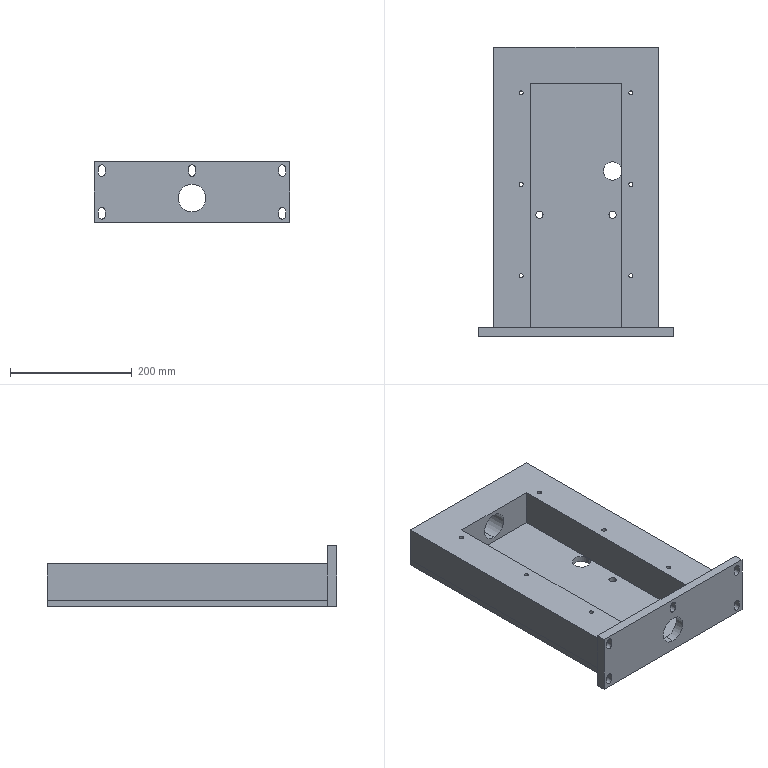Part | SolidWorks | features ICE 4, Cut 3, Extrusion 1, HoleWzd 1 | 3 solids | 81 faces | box 320 x 475 x 100 mm | volume 5416407 mm3 | cylinder 49 | plane 32 | commonest cylinder face diameters 6.8 x24 11 x15 12 x4 45 x4 30 x2